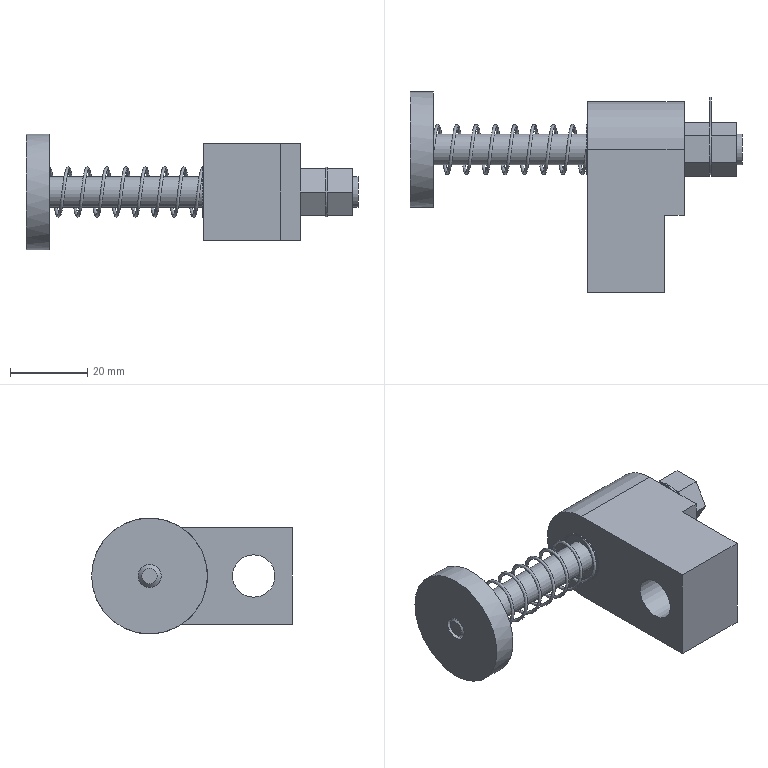Part | NX | features solid 2 | 1 solid | 77 faces | box 86 x 52 x 30 mm | volume 33018 mm3 | plane 60 | cylinder 15 | spline 1 | cone 1 | commonest cylinder face diameters 8 x3 13 x3 12.25 x2 2.5 x1 6 x1 8.1 x1